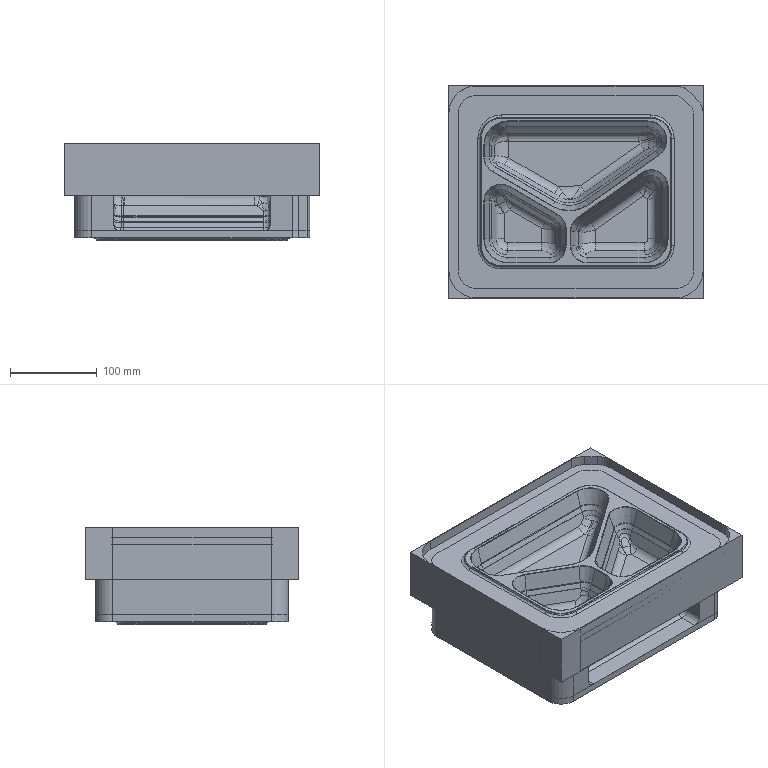NC program | NX | posted with a generic post | part box 295.651 x 246.652 x 112.895 mm
Lines 1 to 1372 of 299251:
N10 G17 G21 G94 G90
(D1 , TOOL : D16R0.8)
N12 T00 M6
N14 G53
N16 G17 G0 G90 X-27.408 Y114.141 S7000 M3 M8
N18 G43 Z210.5 H0
N20 Z61.5
N22 G94 G1 X0. Z60.064 F4500.
N24 X115.613
N26 G2 X124.699 Y110.377 R12.85
N28 G1 X134.877 Y100.2
N30 G2 X138.641 Y91.113 R12.85
N32 G1 Y-91.256
N34 G2 X115.756 Y-114.141 R22.885
N36 G1 X-115.756
N38 G2 X-138.641 Y-91.256 R22.885
N40 G1 Y91.256
N42 G2 X-115.756 Y114.141 R22.885
N44 G1 X0.
N46 Y104.061
N48 X115.613
N50 G2 X117.572 Y103.25 R2.77
N52 G1 X127.749 Y93.072
N54 G2 X128.561 Y91.113 R2.77
N56 G1 Y-91.256
N58 G2 X115.756 Y-104.061 R12.805
N60 G1 X-115.756
N62 G2 X-128.561 Y-91.256 R12.805
N64 G1 Y91.256
N66 G2 X-115.756 Y104.061 R12.805
N68 G1 X0.
N70 Y93.981
N72 X112.585
N74 X118.481 Y88.085
N76 Y-91.256
N78 G2 X115.756 Y-93.981 R2.725
N80 G1 X-115.756
N82 G2 X-118.481 Y-91.256 R2.725
N84 G1 Y91.256
N86 G2 X-115.756 Y93.981 R2.725
N88 G1 X0.
N90 Y83.901
N92 X108.401
N94 Y-83.901
N96 X-108.401
N98 Y83.901
N100 X0.
N102 Y73.821
N104 X98.321
N106 Y-73.821
N108 X-98.321
N110 Y73.821
N112 X0.
N114 Y63.741
N116 X88.241
N118 Y-63.741
N120 X-88.241
N122 Y63.741
N124 X0.
N126 Y53.661
N128 X78.161
N130 Y-53.661
N132 X-78.161
N134 Y53.661
N136 X0.
N138 Y43.581
N140 X68.081
N142 Y-43.581
N144 X-68.081
N146 Y43.581
N148 X0.
N150 Y33.501
N152 X58.001
N154 Y-33.501
N156 X-58.001
N158 Y33.501
N160 X0.
N162 Y23.421
N164 X47.921
N166 Y-23.421
N168 X-47.921
N170 Y23.421
N172 X0.
N174 Y13.341
N176 X37.841
N178 Y-13.341
N180 X-37.841
N182 Y13.341
N184 X0.
N186 Y3.261
N188 X27.761
N190 Y-3.261
N192 X-27.761
N194 Y3.261
N196 X0.
N198 G3 X3.2 Y6.461 R3.2
N200 G1 Z61.064
N202 G0 Z63.5
N204 X-27.408 Y114.076
N206 Z61.064
N208 G1 X0. Z59.627
N210 X115.613
N212 G2 X124.653 Y110.331 R12.785
N214 G1 X134.831 Y100.154
N216 G2 X138.576 Y91.113 R12.785
N218 G1 Y-91.256
N220 G2 X115.756 Y-114.076 R22.82
N222 G1 X-115.756
N224 G2 X-138.576 Y-91.256 R22.82
N226 G1 Y91.256
N228 G2 X-115.756 Y114.076 R22.82
N230 G1 X0.
N232 Y103.996
N234 X115.613
N236 G2 X117.526 Y103.204 R2.705
N238 G1 X127.703 Y93.026
N240 G2 X128.496 Y91.113 R2.705
N242 G1 Y-91.256
N244 G2 X115.756 Y-103.996 R12.74
N246 G1 X-115.756
N248 G2 X-128.496 Y-91.256 R12.74
N250 G1 Y91.256
N252 G2 X-115.756 Y103.996 R12.74
N254 G1 X0.
N256 Y93.916
N258 X112.558
N260 X118.416 Y88.058
N262 Y-91.256
N264 G2 X115.756 Y-93.916 R2.66
N266 G1 X-115.756
N268 G2 X-118.416 Y-91.256 R2.66
N270 G1 Y91.256
N272 G2 X-115.756 Y93.916 R2.66
N274 G1 X0.
N276 Y83.836
N278 X108.336
N280 Y-83.836
N282 X-108.336
N284 Y83.836
N286 X0.
N288 Y73.756
N290 X98.256
N292 Y-73.756
N294 X-98.256
N296 Y73.756
N298 X0.
N300 Y63.676
N302 X88.176
N304 Y-63.676
N306 X-88.176
N308 Y63.676
N310 X0.
N312 Y53.596
N314 X78.096
N316 Y-53.596
N318 X-78.096
N320 Y53.596
N322 X0.
N324 Y43.516
N326 X68.016
N328 Y-43.516
N330 X-68.016
N332 Y43.516
N334 X0.
N336 Y33.436
N338 X57.936
N340 Y-33.436
N342 X-57.936
N344 Y33.436
N346 X0.
N348 Y23.356
N350 X47.856
N352 Y-23.356
N354 X-47.856
N356 Y23.356
N358 X0.
N360 Y13.276
N362 X37.776
N364 Y-13.276
N366 X-37.776
N368 Y13.276
N370 X0.
N372 Y3.196
N374 X27.696
N376 Y-3.196
N378 X-27.696
N380 Y3.196
N382 X0.
N384 G3 X3.2 Y6.396 R3.2
N386 G1 Z60.627
N388 G0 Z63.064
N390 X-27.408 Y114.076
N392 Z60.627
N394 G1 X0. Z59.191
N396 X115.613
N398 G2 X124.653 Y110.331 R12.785
N400 G1 X134.831 Y100.154
N402 G2 X138.576 Y91.113 R12.785
N404 G1 Y-91.256
N406 G2 X115.756 Y-114.076 R22.82
N408 G1 X-115.756
N410 G2 X-138.576 Y-91.256 R22.82
N412 G1 Y91.256
N414 G2 X-115.756 Y114.076 R22.82
N416 G1 X0.
N418 Y103.996
N420 X115.613
N422 G2 X117.526 Y103.204 R2.705
N424 G1 X127.703 Y93.026
N426 G2 X128.496 Y91.113 R2.705
N428 G1 Y-91.256
N430 G2 X115.756 Y-103.996 R12.74
N432 G1 X-115.756
N434 G2 X-128.496 Y-91.256 R12.74
N436 G1 Y91.256
N438 G2 X-115.756 Y103.996 R12.74
N440 G1 X0.
N442 Y93.916
N444 X112.558
N446 X118.416 Y88.058
N448 Y-91.256
N450 G2 X115.756 Y-93.916 R2.66
N452 G1 X-115.756
N454 G2 X-118.416 Y-91.256 R2.66
N456 G1 Y91.256
N458 G2 X-115.756 Y93.916 R2.66
N460 G1 X0.
N462 Y83.836
N464 X108.336
N466 Y-83.836
N468 X-108.336
N470 Y83.836
N472 X0.
N474 Y73.756
N476 X98.256
N478 Y-73.756
N480 X-98.256
N482 Y73.756
N484 X0.
N486 Y63.676
N488 X88.176
N490 Y-63.676
N492 X-88.176
N494 Y63.676
N496 X0.
N498 Y53.596
N500 X78.096
N502 Y-53.596
N504 X-78.096
N506 Y53.596
N508 X0.
N510 Y43.516
N512 X68.016
N514 Y-43.516
N516 X-68.016
N518 Y43.516
N520 X0.
N522 Y33.436
N524 X57.936
N526 Y-33.436
N528 X-57.936
N530 Y33.436
N532 X0.
N534 Y23.356
N536 X47.856
N538 Y-23.356
N540 X-47.856
N542 Y23.356
N544 X0.
N546 Y13.276
N548 X37.776
N550 Y-13.276
N552 X-37.776
N554 Y13.276
N556 X0.
N558 Y3.196
N560 X27.696
N562 Y-3.196
N564 X-27.696
N566 Y3.196
N568 X0.
N570 G3 X3.2 Y6.396 R3.2
N572 G1 Z60.191
N574 G0 Z62.627
N576 X-27.408 Y114.076
N578 Z60.191
N580 G1 X0. Z58.754
N582 X115.613
N584 G2 X124.653 Y110.331 R12.785
N586 G1 X134.831 Y100.154
N588 G2 X138.576 Y91.113 R12.785
N590 G1 Y-91.256
N592 G2 X115.756 Y-114.076 R22.82
N594 G1 X-115.756
N596 G2 X-138.576 Y-91.256 R22.82
N598 G1 Y91.256
N600 G2 X-115.756 Y114.076 R22.82
N602 G1 X0.
N604 Y103.996
N606 X115.613
N608 G2 X117.526 Y103.204 R2.705
N610 G1 X127.703 Y93.026
N612 G2 X128.496 Y91.113 R2.705
N614 G1 Y-91.256
N616 G2 X115.756 Y-103.996 R12.74
N618 G1 X-115.756
N620 G2 X-128.496 Y-91.256 R12.74
N622 G1 Y91.256
N624 G2 X-115.756 Y103.996 R12.74
N626 G1 X0.
N628 Y93.916
N630 X112.558
N632 X118.416 Y88.058
N634 Y-91.256
N636 G2 X115.756 Y-93.916 R2.66
N638 G1 X-115.756
N640 G2 X-118.416 Y-91.256 R2.66
N642 G1 Y91.256
N644 G2 X-115.756 Y93.916 R2.66
N646 G1 X0.
N648 Y83.836
N650 X108.336
N652 Y-83.836
N654 X-108.336
N656 Y83.836
N658 X0.
N660 Y73.756
N662 X98.256
N664 Y-73.756
N666 X-98.256
N668 Y73.756
N670 X0.
N672 Y63.676
N674 X88.176
N676 Y-63.676
N678 X-88.176
N680 Y63.676
N682 X0.
N684 Y53.596
N686 X78.096
N688 Y-53.596
N690 X-78.096
N692 Y53.596
N694 X0.
N696 Y43.516
N698 X68.016
N700 Y-43.516
N702 X-68.016
N704 Y43.516
N706 X0.
N708 Y33.436
N710 X57.936
N712 Y-33.436
N714 X-57.936
N716 Y33.436
N718 X0.
N720 Y23.356
N722 X47.856
N724 Y-23.356
N726 X-47.856
N728 Y23.356
N730 X0.
N732 Y13.276
N734 X37.776
N736 Y-13.276
N738 X-37.776
N740 Y13.276
N742 X0.
N744 Y3.196
N746 X27.696
N748 Y-3.196
N750 X-27.696
N752 Y3.196
N754 X0.
N756 G3 X3.2 Y6.396 R3.2
N758 G1 Z59.754
N760 G0 Z62.191
N762 X-27.408 Y114.076
N764 Z59.754
N766 G1 X0. Z58.318
N768 X115.613
N770 G2 X124.653 Y110.331 R12.785
N772 G1 X134.831 Y100.154
N774 G2 X138.576 Y91.113 R12.785
N776 G1 Y-91.256
N778 G2 X115.756 Y-114.076 R22.82
N780 G1 X-115.756
N782 G2 X-138.576 Y-91.256 R22.82
N784 G1 Y91.256
N786 G2 X-115.756 Y114.076 R22.82
N788 G1 X0.
N790 Y103.996
N792 X115.613
N794 G2 X117.526 Y103.204 R2.705
N796 G1 X127.703 Y93.026
N798 G2 X128.496 Y91.113 R2.705
N800 G1 Y-91.256
N802 G2 X115.756 Y-103.996 R12.74
N804 G1 X-115.756
N806 G2 X-128.496 Y-91.256 R12.74
N808 G1 Y91.256
N810 G2 X-115.756 Y103.996 R12.74
N812 G1 X0.
N814 Y93.916
N816 X112.558
N818 X118.416 Y88.058
N820 Y-91.256
N822 G2 X115.756 Y-93.916 R2.66
N824 G1 X-115.756
N826 G2 X-118.416 Y-91.256 R2.66
N828 G1 Y91.256
N830 G2 X-115.756 Y93.916 R2.66
N832 G1 X0.
N834 Y83.836
N836 X108.336
N838 Y-83.836
N840 X-108.336
N842 Y83.836
N844 X0.
N846 Y73.756
N848 X98.256
N850 Y-73.756
N852 X-98.256
N854 Y73.756
N856 X0.
N858 Y63.676
N860 X88.176
N862 Y-63.676
N864 X-88.176
N866 Y63.676
N868 X0.
N870 Y53.596
N872 X78.096
N874 Y-53.596
N876 X-78.096
N878 Y53.596
N880 X0.
N882 Y43.516
N884 X68.016
N886 Y-43.516
N888 X-68.016
N890 Y43.516
N892 X0.
N894 Y33.436
N896 X57.936
N898 Y-33.436
N900 X-57.936
N902 Y33.436
N904 X0.
N906 Y23.356
N908 X47.856
N910 Y-23.356
N912 X-47.856
N914 Y23.356
N916 X0.
N918 Y13.276
N920 X37.776
N922 Y-13.276
N924 X-37.776
N926 Y13.276
N928 X0.
N930 Y3.196
N932 X27.696
N934 Y-3.196
N936 X-27.696
N938 Y3.196
N940 X0.
N942 G3 X3.2 Y6.396 R3.2
N944 G1 Z59.318
N946 G0 Z61.754
N948 X-27.408 Y114.076
N950 Z59.318
N952 G1 X0. Z57.882
N954 X115.613
N956 G2 X124.653 Y110.331 R12.785
N958 G1 X134.831 Y100.154
N960 G2 X138.576 Y91.113 R12.785
N962 G1 Y-91.256
N964 G2 X115.756 Y-114.076 R22.82
N966 G1 X-115.756
N968 G2 X-138.576 Y-91.256 R22.82
N970 G1 Y91.256
N972 G2 X-115.756 Y114.076 R22.82
N974 G1 X0.
N976 Y103.996
N978 X115.613
N980 G2 X117.526 Y103.204 R2.705
N982 G1 X127.703 Y93.026
N984 G2 X128.496 Y91.113 R2.705
N986 G1 Y-91.256
N988 G2 X115.756 Y-103.996 R12.74
N990 G1 X-115.756
N992 G2 X-128.496 Y-91.256 R12.74
N994 G1 Y91.256
N996 G2 X-115.756 Y103.996 R12.74
N998 G1 X0.
N1000 Y93.916
N1002 X112.558
N1004 X118.416 Y88.058
N1006 Y-91.256
N1008 G2 X115.756 Y-93.916 R2.66
N1010 G1 X-115.756
N1012 G2 X-118.416 Y-91.256 R2.66
N1014 G1 Y91.256
N1016 G2 X-115.756 Y93.916 R2.66
N1018 G1 X0.
N1020 Y83.836
N1022 X108.336
N1024 Y-83.836
N1026 X-108.336
N1028 Y83.836
N1030 X0.
N1032 Y73.756
N1034 X98.256
N1036 Y-73.756
N1038 X-98.256
N1040 Y73.756
N1042 X0.
N1044 Y63.676
N1046 X88.176
N1048 Y-63.676
N1050 X-88.176
N1052 Y63.676
N1054 X0.
N1056 Y53.596
N1058 X78.096
N1060 Y-53.596
N1062 X-78.096
N1064 Y53.596
N1066 X0.
N1068 Y43.516
N1070 X68.016
N1072 Y-43.516
N1074 X-68.016
N1076 Y43.516
N1078 X0.
N1080 Y33.436
N1082 X57.936
N1084 Y-33.436
N1086 X-57.936
N1088 Y33.436
N1090 X0.
N1092 Y23.356
N1094 X47.856
N1096 Y-23.356
N1098 X-47.856
N1100 Y23.356
N1102 X0.
N1104 Y13.276
N1106 X37.776
N1108 Y-13.276
N1110 X-37.776
N1112 Y13.276
N1114 X0.
N1116 Y3.196
N1118 X27.696
N1120 Y-3.196
N1122 X-27.696
N1124 Y3.196
N1126 X0.
N1128 G3 X3.2 Y6.396 R3.2
N1130 G1 Z58.882
N1132 G0 Z61.318
N1134 X-27.408 Y114.076
N1136 Z58.882
N1138 G1 X0. Z57.445
N1140 X115.613
N1142 G2 X124.653 Y110.331 R12.785
N1144 G1 X134.831 Y100.154
N1146 G2 X138.576 Y91.113 R12.785
N1148 G1 Y-91.256
N1150 G2 X115.756 Y-114.076 R22.82
N1152 G1 X-115.756
N1154 G2 X-138.576 Y-91.256 R22.82
N1156 G1 Y91.256
N1158 G2 X-115.756 Y114.076 R22.82
N1160 G1 X0.
N1162 Y103.996
N1164 X115.613
N1166 G2 X117.526 Y103.204 R2.705
N1168 G1 X127.703 Y93.026
N1170 G2 X128.496 Y91.113 R2.705
N1172 G1 Y-91.256
N1174 G2 X115.756 Y-103.996 R12.74
N1176 G1 X-115.756
N1178 G2 X-128.496 Y-91.256 R12.74
N1180 G1 Y91.256
N1182 G2 X-115.756 Y103.996 R12.74
N1184 G1 X0.
N1186 Y93.916
N1188 X112.558
N1190 X118.416 Y88.058
N1192 Y-91.256
N1194 G2 X115.756 Y-93.916 R2.66
N1196 G1 X-115.756
N1198 G2 X-118.416 Y-91.256 R2.66
N1200 G1 Y91.256
N1202 G2 X-115.756 Y93.916 R2.66
N1204 G1 X0.
N1206 Y83.836
N1208 X108.336
N1210 Y-83.836
N1212 X-108.336
N1214 Y83.836
N1216 X0.
N1218 Y73.756
N1220 X98.256
N1222 Y-73.756
N1224 X-98.256
N1226 Y73.756
N1228 X0.
N1230 Y63.676
N1232 X88.176
N1234 Y-63.676
N1236 X-88.176
N1238 Y63.676
N1240 X0.
N1242 Y53.596
N1244 X78.096
N1246 Y-53.596
N1248 X-78.096
N1250 Y53.596
N1252 X0.
N1254 Y43.516
N1256 X68.016
N1258 Y-43.516
N1260 X-68.016
N1262 Y43.516
N1264 X0.
N1266 Y33.436
N1268 X57.936
N1270 Y-33.436
N1272 X-57.936
N1274 Y33.436
N1276 X0.
N1278 Y23.356
N1280 X47.856
N1282 Y-23.356
N1284 X-47.856
N1286 Y23.356
N1288 X0.
N1290 Y13.276
N1292 X37.776
N1294 Y-13.276
N1296 X-37.776
N1298 Y13.276
N1300 X0.
N1302 Y3.196
N1304 X27.696
N1306 Y-3.196
N1308 X-27.696
N1310 Y3.196
N1312 X0.
N1314 G3 X3.2 Y6.396 R3.2
N1316 G1 Z58.445
N1318 G0 Z60.882
N1320 X-27.408 Y114.076
N1322 Z58.445
N1324 G1 X0. Z57.009
N1326 X115.613
N1328 G2 X124.653 Y110.331 R12.785
N1330 G1 X134.831 Y100.154
N1332 G2 X138.576 Y91.113 R12.785
N1334 G1 Y-91.256
N1336 G2 X115.756 Y-114.076 R22.82
N1338 G1 X-115.756
N1340 G2 X-138.576 Y-91.256 R22.82
N1342 G1 Y91.256
N1344 G2 X-115.756 Y114.076 R22.82
N1346 G1 X0.
N1348 Y103.996
N1350 X115.613
N1352 G2 X117.526 Y103.204 R2.705
N1354 G1 X127.703 Y93.026
N1356 G2 X128.496 Y91.113 R2.705
N1358 G1 Y-91.256
N1360 G2 X115.756 Y-103.996 R12.74
N1362 G1 X-115.756
N1364 G2 X-128.496 Y-91.256 R12.74
N1366 G1 Y91.256
N1368 G2 X-115.756 Y103.996 R12.74
N1370 G1 X0.
N1372 Y93.916
N1374 X112.558
N1376 X118.416 Y88.058
N1378 Y-91.256
N1380 G2 X115.756 Y-93.916 R2.66
N1382 G1 X-115.756
N1384 G2 X-118.416 Y-91.256 R2.66
N1386 G1 Y91.256
N1388 G2 X-115.756 Y93.916 R2.66
N1390 G1 X0.
N1392 Y83.836
N1394 X108.336
N1396 Y-83.836
N1398 X-108.336
N1400 Y83.836
N1402 X0.
N1404 Y73.756
N1406 X98.256
N1408 Y-73.756
N1410 X-98.256
N1412 Y73.756
N1414 X0.
N1416 Y63.676
N1418 X88.176
N1420 Y-63.676
N1422 X-88.176
N1424 Y63.676
N1426 X0.
N1428 Y53.596
N1430 X78.096
N1432 Y-53.596
N1434 X-78.096
N1436 Y53.596
N1438 X0.
N1440 Y43.516
N1442 X68.016
N1444 Y-43.516
N1446 X-68.016
N1448 Y43.516
N1450 X0.
N1452 Y33.436
N1454 X57.936
N1456 Y-33.436
N1458 X-57.936
N1460 Y33.436
N1462 X0.
N1464 Y23.356
N1466 X47.856
N1468 Y-23.356
N1470 X-47.856
N1472 Y23.356
N1474 X0.
N1476 Y13.276
N1478 X37.776
N1480 Y-13.276
N1482 X-37.776
N1484 Y13.276
N1486 X0.
N1488 Y3.196
N1490 X27.696
N1492 Y-3.196
N1494 X-27.696
N1496 Y3.196
N1498 X0.
N1500 G3 X3.2 Y6.396 R3.2
N1502 G1 Z58.009
N1504 G0 Z60.445
N1506 X-27.408 Y114.076
N1508 Z58.009
N1510 G1 X0. Z56.573
N1512 X115.613
N1514 G2 X124.653 Y110.331 R12.785
N1516 G1 X134.831 Y100.154
N1518 G2 X138.576 Y91.113 R12.785
N1520 G1 Y-91.256
N1522 G2 X115.756 Y-114.076 R22.82
N1524 G1 X-115.756
N1526 G2 X-138.576 Y-91.256 R22.82
N1528 G1 Y91.256
N1530 G2 X-115.756 Y114.076 R22.82
N1532 G1 X0.
N1534 Y103.996
N1536 X115.613
N1538 G2 X117.526 Y103.204 R2.705
N1540 G1 X127.703 Y93.026
N1542 G2 X128.496 Y91.113 R2.705
N1544 G1 Y-91.256
N1546 G2 X115.756 Y-103.996 R12.74
N1548 G1 X-115.756
N1550 G2 X-128.496 Y-91.256 R12.74
N1552 G1 Y91.256
N1554 G2 X-115.756 Y103.996 R12.74
N1556 G1 X0.
N1558 Y93.916
N1560 X112.558
N1562 X118.416 Y88.058
N1564 Y-91.256
N1566 G2 X115.756 Y-93.916 R2.66
N1568 G1 X-115.756
N1570 G2 X-118.416 Y-91.256 R2.66
N1572 G1 Y91.256
N1574 G2 X-115.756 Y93.916 R2.66
N1576 G1 X0.
N1578 Y83.836
N1580 X108.336
N1582 Y-83.836
N1584 X-108.336
N1586 Y83.836
N1588 X0.
N1590 Y73.756
N1592 X98.256
N1594 Y-73.756
N1596 X-98.256
N1598 Y73.756
N1600 X0.
N1602 Y63.676
N1604 X88.176
N1606 Y-63.676
N1608 X-88.176
N1610 Y63.676
N1612 X0.
N1614 Y53.596
N1616 X78.096
N1618 Y-53.596
N1620 X-78.096
N1622 Y53.596
N1624 X0.
N1626 Y43.516
N1628 X68.016
N1630 Y-43.516
N1632 X-68.016
N1634 Y43.516
N1636 X0.
N1638 Y33.436
N1640 X57.936
N1642 Y-33.436
N1644 X-57.936
N1646 Y33.436
N1648 X0.
N1650 Y23.356
N1652 X47.856
N1654 Y-23.356
N1656 X-47.856
N1658 Y23.356
N1660 X0.
N1662 Y13.276
N1664 X37.776
N1666 Y-13.276
N1668 X-37.776
N1670 Y13.276
N1672 X0.
N1674 Y3.196
N1676 X27.696
N1678 Y-3.196
N1680 X-27.696
N1682 Y3.196
N1684 X0.
N1686 G3 X3.2 Y6.396 R3.2
N1688 G1 Z57.573
N1690 G0 Z60.009
N1692 X-27.408 Y114.076
N1694 Z57.573
N1696 G1 X0. Z56.136
N1698 X115.613
N1700 G2 X124.653 Y110.331 R12.785
N1702 G1 X134.831 Y100.154
N1704 G2 X138.576 Y91.113 R12.785
N1706 G1 Y-91.256
N1708 G2 X115.756 Y-114.076 R22.82
N1710 G1 X-115.756
N1712 G2 X-138.576 Y-91.256 R22.82
N1714 G1 Y91.256
N1716 G2 X-115.756 Y114.076 R22.82
N1718 G1 X0.
N1720 Y103.996
N1722 X115.613
N1724 G2 X117.526 Y103.204 R2.705
N1726 G1 X127.703 Y93.026
N1728 G2 X128.496 Y91.113 R2.705
N1730 G1 Y-91.256
N1732 G2 X115.756 Y-103.996 R12.74
N1734 G1 X-115.756
N1736 G2 X-128.496 Y-91.256 R12.74
N1738 G1 Y91.256
N1740 G2 X-115.756 Y103.996 R12.74
N1742 G1 X0.
N1744 Y93.916
N1746 X112.558
N1748 X118.416 Y88.058
N1750 Y-91.256
N1752 G2 X115.756 Y-93.916 R2.66
N1754 G1 X-115.756
N1756 G2 X-118.416 Y-91.256 R2.66
N1758 G1 Y91.256
N1760 G2 X-115.756 Y93.916 R2.66
N1762 G1 X0.
N1764 Y83.836
N1766 X108.336
N1768 Y-83.836
N1770 X-108.336
N1772 Y83.836
N1774 X0.
N1776 Y73.756
N1778 X98.256
N1780 Y-73.756
N1782 X-98.256
N1784 Y73.756
N1786 X0.
N1788 Y63.676
N1790 X88.176
N1792 Y-63.676
N1794 X-88.176
N1796 Y63.676
N1798 X0.
N1800 Y53.596
N1802 X78.096
N1804 Y-53.596
N1806 X-78.096
N1808 Y53.596
N1810 X0.
N1812 Y43.516
N1814 X68.016
N1816 Y-43.516
N1818 X-68.016
N1820 Y43.516
N1822 X0.
N1824 Y33.436
N1826 X57.936
N1828 Y-33.436
N1830 X-57.936
N1832 Y33.436
N1834 X0.
N1836 Y23.356
N1838 X47.856
N1840 Y-23.356
N1842 X-47.856
N1844 Y23.356
N1846 X0.
N1848 Y13.276
N1850 X37.776
N1852 Y-13.276
N1854 X-37.776
N1856 Y13.276
N1858 X0.
N1860 Y3.196
N1862 X27.696
N1864 Y-3.196
N1866 X-27.696
N1868 Y3.196
N1870 X0.
N1872 G3 X3.2 Y6.396 R3.2
N1874 G1 Z57.136
N1876 G0 Z59.573
N1878 X-27.408 Y114.076
N1880 Z57.136
N1882 G1 X0. Z55.7
N1884 X115.613
N1886 G2 X124.653 Y110.331 R12.785
N1888 G1 X134.831 Y100.154
N1890 G2 X138.576 Y91.113 R12.785
N1892 G1 Y-91.256
N1894 G2 X115.756 Y-114.076 R22.82
N1896 G1 X-115.756
N1898 G2 X-138.576 Y-91.256 R22.82
N1900 G1 Y91.256
N1902 G2 X-115.756 Y114.076 R22.82
N1904 G1 X0.
N1906 Y103.996
N1908 X115.613
N1910 G2 X117.526 Y103.204 R2.705
N1912 G1 X127.703 Y93.026
N1914 G2 X128.496 Y91.113 R2.705
N1916 G1 Y-91.256
N1918 G2 X115.756 Y-103.996 R12.74
N1920 G1 X-115.756
N1922 G2 X-128.496 Y-91.256 R12.74
N1924 G1 Y91.256
N1926 G2 X-115.756 Y103.996 R12.74
N1928 G1 X0.
N1930 Y93.916
N1932 X112.558
N1934 X118.416 Y88.058
N1936 Y-91.256
N1938 G2 X115.756 Y-93.916 R2.66
N1940 G1 X-115.756
N1942 G2 X-118.416 Y-91.256 R2.66
N1944 G1 Y91.256
N1946 G2 X-115.756 Y93.916 R2.66
N1948 G1 X0.
N1950 Y83.836
N1952 X108.336
N1954 Y-83.836
N1956 X-108.336
N1958 Y83.836
N1960 X0.
N1962 Y73.756
N1964 X98.256
N1966 Y-73.756
N1968 X-98.256
N1970 Y73.756
N1972 X0.
N1974 Y63.676
N1976 X88.176
N1978 Y-63.676
N1980 X-88.176
N1982 Y63.676
N1984 X0.
N1986 Y53.596
N1988 X78.096
N1990 Y-53.596
N1992 X-78.096
N1994 Y53.596
N1996 X0.
N1998 Y43.516
N2000 X68.016
N2002 Y-43.516
N2004 X-68.016
N2006 Y43.516
N2008 X0.
N2010 Y33.436
N2012 X57.936
N2014 Y-33.436
N2016 X-57.936
N2018 Y33.436
N2020 X0.
N2022 Y23.356
N2024 X47.856
N2026 Y-23.356
N2028 X-47.856
N2030 Y23.356
N2032 X0.
N2034 Y13.276
N2036 X37.776
N2038 Y-13.276
N2040 X-37.776
N2042 Y13.276
N2044 X0.
N2046 Y3.196
N2048 X27.696
N2050 Y-3.196
N2052 X-27.696
N2054 Y3.196
N2056 X0.
N2058 G3 X3.2 Y6.396 R3.2
N2060 G1 Z56.7
N2062 G0 Z59.136
N2064 X-27.408 Y114.076
N2066 Z56.7
N2068 G1 X0. Z55.263
N2070 X115.613
N2072 G2 X124.653 Y110.331 R12.785
N2074 G1 X134.831 Y100.154
N2076 G2 X138.576 Y91.113 R12.785
N2078 G1 Y-91.256
N2080 G2 X115.756 Y-114.076 R22.82
N2082 G1 X-115.756
N2084 G2 X-138.576 Y-91.256 R22.82
N2086 G1 Y91.256
N2088 G2 X-115.756 Y114.076 R22.82
N2090 G1 X0.
N2092 Y103.996
N2094 X115.613
N2096 G2 X117.526 Y103.204 R2.705
N2098 G1 X127.703 Y93.026
N2100 G2 X128.496 Y91.113 R2.705
N2102 G1 Y-91.256
N2104 G2 X115.756 Y-103.996 R12.74
N2106 G1 X-115.756
N2108 G2 X-128.496 Y-91.256 R12.74
N2110 G1 Y91.256
N2112 G2 X-115.756 Y103.996 R12.74
N2114 G1 X0.
N2116 Y93.916
N2118 X112.558
N2120 X118.416 Y88.058
N2122 Y-91.256
N2124 G2 X115.756 Y-93.916 R2.66
N2126 G1 X-115.756
N2128 G2 X-118.416 Y-91.256 R2.66
N2130 G1 Y91.256
N2132 G2 X-115.756 Y93.916 R2.66
N2134 G1 X0.
N2136 Y83.836
N2138 X108.336
N2140 Y-83.836
N2142 X-108.336
N2144 Y83.836
N2146 X0.
N2148 Y73.756
N2150 X98.256
N2152 Y-73.756
N2154 X-98.256
N2156 Y73.756
N2158 X0.
N2160 Y63.676
N2162 X88.176
N2164 Y-63.676
N2166 X-88.176
N2168 Y63.676
N2170 X0.
N2172 Y53.596
N2174 X78.096
N2176 Y-53.596
N2178 X-78.096
N2180 Y53.596
N2182 X0.
N2184 Y43.516
N2186 X68.016
N2188 Y-43.516
N2190 X-68.016
N2192 Y43.516
N2194 X0.
N2196 Y33.436
N2198 X57.936
N2200 Y-33.436
N2202 X-57.936
N2204 Y33.436
N2206 X0.
N2208 Y23.356
N2210 X47.856
N2212 Y-23.356
N2214 X-47.856
N2216 Y23.356
N2218 X0.
N2220 Y13.276
N2222 X37.776
N2224 Y-13.276
N2226 X-37.776
N2228 Y13.276
N2230 X0.
N2232 Y3.196
N2234 X27.696
N2236 Y-3.196
N2238 X-27.696
N2240 Y3.196
N2242 X0.
N2244 G3 X3.2 Y6.396 R3.2
N2246 G1 Z56.263
N2248 G0 Z58.7
N2250 X-27.408 Y114.076
N2252 Z56.263
N2254 G1 X0. Z54.827
N2256 X115.613
N2258 G2 X124.653 Y110.331 R12.785
N2260 G1 X134.831 Y100.154
N2262 G2 X138.576 Y91.113 R12.785
N2264 G1 Y-91.256
N2266 G2 X115.756 Y-114.076 R22.82
N2268 G1 X-115.756
N2270 G2 X-138.576 Y-91.256 R22.82
N2272 G1 Y91.256
N2274 G2 X-115.756 Y114.076 R22.82
N2276 G1 X0.
N2278 Y103.996
N2280 X115.613
N2282 G2 X117.526 Y103.204 R2.705
N2284 G1 X127.703 Y93.026
N2286 G2 X128.496 Y91.113 R2.705
N2288 G1 Y-91.256
N2290 G2 X115.756 Y-103.996 R12.74
N2292 G1 X-115.756
N2294 G2 X-128.496 Y-91.256 R12.74
N2296 G1 Y91.256
N2298 G2 X-115.756 Y103.996 R12.74
N2300 G1 X0.
N2302 Y93.916
N2304 X112.558
N2306 X118.416 Y88.058
N2308 Y-91.256
N2310 G2 X115.756 Y-93.916 R2.66
N2312 G1 X-115.756
N2314 G2 X-118.416 Y-91.256 R2.66
N2316 G1 Y91.256
N2318 G2 X-115.756 Y93.916 R2.66
N2320 G1 X0.
N2322 Y83.836
N2324 X108.336
N2326 Y-83.836
N2328 X-108.336
N2330 Y83.836
N2332 X0.
N2334 Y73.756
N2336 X98.256
N2338 Y-73.756
N2340 X-98.256
N2342 Y73.756
N2344 X0.
N2346 Y63.676
N2348 X88.176
N2350 Y-63.676
N2352 X-88.176
N2354 Y63.676
N2356 X0.
N2358 Y53.596
N2360 X78.096
N2362 Y-53.596
N2364 X-78.096
N2366 Y53.596
N2368 X0.
N2370 Y43.516
N2372 X68.016
N2374 Y-43.516
N2376 X-68.016
N2378 Y43.516
N2380 X0.
N2382 Y33.436
N2384 X57.936
N2386 Y-33.436
N2388 X-57.936
N2390 Y33.436
N2392 X0.
N2394 Y23.356
N2396 X47.856
N2398 Y-23.356
N2400 X-47.856
N2402 Y23.356
N2404 X0.
N2406 Y13.276
N2408 X37.776
N2410 Y-13.276
N2412 X-37.776
N2414 Y13.276
N2416 X0.
N2418 Y3.196
N2420 X27.696
N2422 Y-3.196
N2424 X-27.696
N2426 Y3.196
N2428 X0.
N2430 G3 X3.2 Y6.396 R3.2
N2432 G1 Z55.827
N2434 G0 Z58.263
N2436 X-27.408 Y114.076
N2438 Z55.827
N2440 G1 X0. Z54.391
N2442 X115.613
N2444 G2 X124.653 Y110.331 R12.785
N2446 G1 X134.831 Y100.154
N2448 G2 X138.576 Y91.113 R12.785
N2450 G1 Y-91.256
N2452 G2 X115.756 Y-114.076 R22.82
N2454 G1 X-115.756
N2456 G2 X-138.576 Y-91.256 R22.82
N2458 G1 Y91.256
N2460 G2 X-115.756 Y114.076 R22.82
N2462 G1 X0.
N2464 Y103.996
N2466 X115.613
N2468 G2 X117.526 Y103.204 R2.705
N2470 G1 X127.703 Y93.026
N2472 G2 X128.496 Y91.113 R2.705
N2474 G1 Y-91.256
N2476 G2 X115.756 Y-103.996 R12.74
N2478 G1 X-115.756
N2480 G2 X-128.496 Y-91.256 R12.74
N2482 G1 Y91.256
N2484 G2 X-115.756 Y103.996 R12.74
N2486 G1 X0.
N2488 Y93.916
N2490 X112.558
N2492 X118.416 Y88.058
N2494 Y-91.256
N2496 G2 X115.756 Y-93.916 R2.66
N2498 G1 X-115.756
N2500 G2 X-118.416 Y-91.256 R2.66
N2502 G1 Y91.256
N2504 G2 X-115.756 Y93.916 R2.66
N2506 G1 X0.
N2508 Y83.836
N2510 X108.336
N2512 Y-83.836
N2514 X-108.336
N2516 Y83.836
N2518 X0.
N2520 Y73.756
N2522 X98.256
N2524 Y-73.756
N2526 X-98.256
N2528 Y73.756
N2530 X0.
N2532 Y63.676
N2534 X88.176
N2536 Y-63.676
N2538 X-88.176
N2540 Y63.676
N2542 X0.
N2544 Y53.596
N2546 X78.096
N2548 Y-53.596
N2550 X-78.096
N2552 Y53.596
N2554 X0.
N2556 Y43.516
N2558 X68.016
N2560 Y-43.516
N2562 X-68.016
N2564 Y43.516
N2566 X0.
N2568 Y33.436
N2570 X57.936
N2572 Y-33.436
N2574 X-57.936
N2576 Y33.436
N2578 X0.
N2580 Y23.356
N2582 X47.856
N2584 Y-23.356
N2586 X-47.856
N2588 Y23.356
N2590 X0.
N2592 Y13.276
N2594 X37.776
N2596 Y-13.276
N2598 X-37.776
N2600 Y13.276
N2602 X0.
N2604 Y3.196
N2606 X27.696
N2608 Y-3.196
N2610 X-27.696
N2612 Y3.196
N2614 X0.
N2616 G3 X3.2 Y6.396 R3.2
N2618 G1 Z55.391
N2620 G0 Z57.827
N2622 X-27.408 Y114.076
N2624 Z55.391
N2626 G1 X0. Z53.954
N2628 X115.613
N2630 G2 X124.653 Y110.331 R12.785
N2632 G1 X134.831 Y100.154
N2634 G2 X138.576 Y91.113 R12.785
N2636 G1 Y-91.256
N2638 G2 X115.756 Y-114.076 R22.82
N2640 G1 X-115.756
N2642 G2 X-138.576 Y-91.256 R22.82
N2644 G1 Y91.256
N2646 G2 X-115.756 Y114.076 R22.82
N2648 G1 X0.
N2650 Y103.996
N2652 X115.613
N2654 G2 X117.526 Y103.204 R2.705
N2656 G1 X127.703 Y93.026
N2658 G2 X128.496 Y91.113 R2.705
N2660 G1 Y-91.256
N2662 G2 X115.756 Y-103.996 R12.74
N2664 G1 X-115.756
N2666 G2 X-128.496 Y-91.256 R12.74
N2668 G1 Y91.256
N2670 G2 X-115.756 Y103.996 R12.74
N2672 G1 X0.
N2674 Y93.916
N2676 X112.558
N2678 X118.416 Y88.058
N2680 Y-91.256
N2682 G2 X115.756 Y-93.916 R2.66
N2684 G1 X-115.756
N2686 G2 X-118.416 Y-91.256 R2.66
N2688 G1 Y91.256
N2690 G2 X-115.756 Y93.916 R2.66
N2692 G1 X0.
N2694 Y83.836
N2696 X108.336
N2698 Y-83.836
N2700 X-108.336
N2702 Y83.836
N2704 X0.
N2706 Y73.756
N2708 X98.256
N2710 Y-73.756
N2712 X-98.256
N2714 Y73.756
N2716 X0.
N2718 Y63.676
N2720 X88.176
N2722 Y-63.676
N2724 X-88.176
N2726 Y63.676
N2728 X0.
N2730 Y53.596
N2732 X78.096
N2734 Y-53.596
N2736 X-78.096
N2738 Y53.596
N2740 X0.
N2742 Y43.516